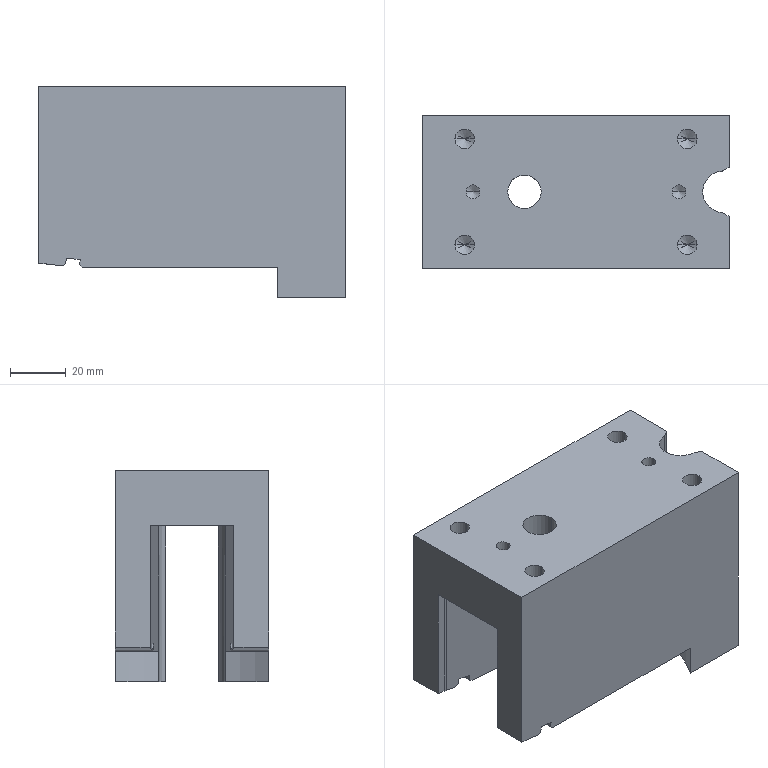Part | 1 solid | 68 faces | box 110 x 55 x 76 mm | volume 272005 mm3 | plane 33 | cylinder 23 | cone 12 | commonest cylinder face diameters 7 x8 20 x6 5 x4 12 x2 98 x2 15 x1